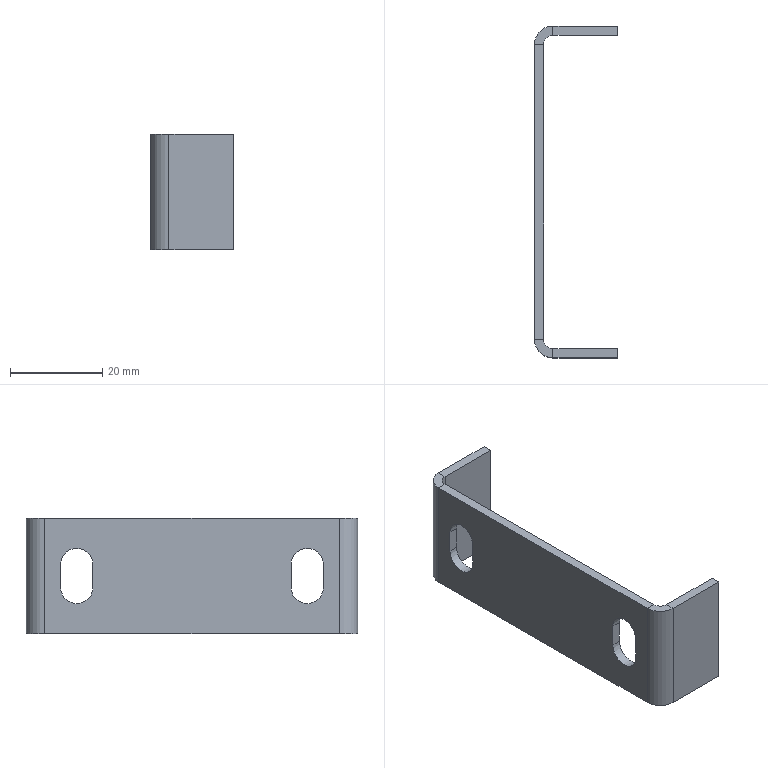Part | SolidWorks | features FlatPattern 1, ICE 1, SMBaseFlange 1, SheetMetal 1 | 1 solid | 32 faces | box 18 x 72 x 25 mm | volume 4777 mm3 | plane 22 | cylinder 10 | commonest cylinder face diameters 7 x6 4 x2 8 x2
STEP:
#1=CARTESIAN_POINT('',(2.,61.,18.5));
#2=VERTEX_POINT('',#1);
#3=CARTESIAN_POINT('',(2.,64.5,15.));
#4=VERTEX_POINT('',#3);
#5=CARTESIAN_POINT('',(2.,61.,15.));
#6=DIRECTION('',(-1.,0.,0.));
#7=DIRECTION('',(0.,0.,1.));
#8=AXIS2_PLACEMENT_3D('',#5,#6,#7);
#9=CIRCLE('',#8,3.5);
#10=EDGE_CURVE('',#2,#4,#9,.T.);
#11=ORIENTED_EDGE('',*,*,#10,.F.);
#12=CARTESIAN_POINT('',(0.,61.,18.5));
#13=VERTEX_POINT('',#12);
#14=CARTESIAN_POINT('',(2.,61.,18.5));
#15=DIRECTION('',(-1.,0.,0.));
#16=VECTOR('',#15,1000.);
#17=LINE('',#14,#16);
#18=EDGE_CURVE('',#2,#13,#17,.T.);
#19=ORIENTED_EDGE('',*,*,#18,.T.);
#20=CARTESIAN_POINT('',(0.,64.5,15.));
#21=VERTEX_POINT('',#20);
#22=CARTESIAN_POINT('',(0.,61.,15.));
#23=DIRECTION('',(-1.,0.,0.));
#24=DIRECTION('',(0.,0.,1.));
#25=AXIS2_PLACEMENT_3D('',#22,#23,#24);
#26=CIRCLE('',#25,3.5);
#27=EDGE_CURVE('',#13,#21,#26,.T.);
#28=ORIENTED_EDGE('',*,*,#27,.T.);
#29=CARTESIAN_POINT('',(2.,64.5,15.));
#30=DIRECTION('',(-1.,0.,0.));
#31=VECTOR('',#30,1000.);
#32=LINE('',#29,#31);
#33=EDGE_CURVE('',#4,#21,#32,.T.);
#34=ORIENTED_EDGE('',*,*,#33,.F.);
#35=EDGE_LOOP('',(#11,#19,#28,#34));
#36=FACE_OUTER_BOUND('',#35,.T.);
#37=CARTESIAN_POINT('',(2.,61.,15.));
#38=DIRECTION('',(-1.,0.,0.));
#39=DIRECTION('',(0.,0.,1.));
#40=AXIS2_PLACEMENT_3D('',#37,#38,#39);
#41=CYLINDRICAL_SURFACE('',#40,3.5);
#42=ADVANCED_FACE('',(#36),#41,.F.);
#43=CARTESIAN_POINT('',(2.,11.,18.5));
#44=VERTEX_POINT('',#43);
#45=CARTESIAN_POINT('',(2.,14.5,15.));
#46=VERTEX_POINT('',#45);
#47=CARTESIAN_POINT('',(2.,11.,15.));
#48=DIRECTION('',(-1.,0.,0.));
#49=DIRECTION('',(0.,0.,-1.));
#50=AXIS2_PLACEMENT_3D('',#47,#48,#49);
#51=CIRCLE('',#50,3.5);
#52=EDGE_CURVE('',#44,#46,#51,.T.);
#53=ORIENTED_EDGE('',*,*,#52,.F.);
#54=CARTESIAN_POINT('',(0.,11.,18.5));
#55=VERTEX_POINT('',#54);
#56=CARTESIAN_POINT('',(2.,11.,18.5));
#57=DIRECTION('',(-1.,0.,0.));
#58=VECTOR('',#57,1000.);
#59=LINE('',#56,#58);
#60=EDGE_CURVE('',#44,#55,#59,.T.);
#61=ORIENTED_EDGE('',*,*,#60,.T.);
#62=CARTESIAN_POINT('',(0.,14.5,15.));
#63=VERTEX_POINT('',#62);
#64=CARTESIAN_POINT('',(0.,11.,15.));
#65=DIRECTION('',(-1.,0.,0.));
#66=DIRECTION('',(0.,0.,-1.));
#67=AXIS2_PLACEMENT_3D('',#64,#65,#66);
#68=CIRCLE('',#67,3.5);
#69=EDGE_CURVE('',#55,#63,#68,.T.);
#70=ORIENTED_EDGE('',*,*,#69,.T.);
#71=CARTESIAN_POINT('',(2.,14.5,15.));
#72=DIRECTION('',(-1.,0.,0.));
#73=VECTOR('',#72,1000.);
#74=LINE('',#71,#73);
#75=EDGE_CURVE('',#46,#63,#74,.T.);
#76=ORIENTED_EDGE('',*,*,#75,.F.);
#77=EDGE_LOOP('',(#53,#61,#70,#76));
#78=FACE_OUTER_BOUND('',#77,.T.);
#79=CARTESIAN_POINT('',(2.,11.,15.));
#80=DIRECTION('',(-1.,0.,0.));
#81=DIRECTION('',(0.,0.,1.));
#82=AXIS2_PLACEMENT_3D('',#79,#80,#81);
#83=CYLINDRICAL_SURFACE('',#82,3.5);
#84=ADVANCED_FACE('',(#78),#83,.F.);
#85=CARTESIAN_POINT('',(4.,72.,25.));
#86=VERTEX_POINT('',#85);
#87=CARTESIAN_POINT('',(4.,70.,25.));
#88=VERTEX_POINT('',#87);
#89=CARTESIAN_POINT('',(4.,72.,25.));
#90=DIRECTION('',(0.,-1.,0.));
#91=VECTOR('',#90,1000.);
#92=LINE('',#89,#91);
#93=EDGE_CURVE('',#86,#88,#92,.T.);
#94=ORIENTED_EDGE('',*,*,#93,.F.);
#95=CARTESIAN_POINT('',(0.,68.,25.));
#96=VERTEX_POINT('',#95);
#97=CARTESIAN_POINT('',(4.,68.,25.));
#98=DIRECTION('',(0.,0.,-1.));
#99=DIRECTION('',(-1.,0.,0.));
#100=AXIS2_PLACEMENT_3D('',#97,#98,#99);
#101=CIRCLE('',#100,4.);
#102=EDGE_CURVE('',#96,#86,#101,.T.);
#103=ORIENTED_EDGE('',*,*,#102,.F.);
#104=CARTESIAN_POINT('',(2.,68.,25.));
#105=VERTEX_POINT('',#104);
#106=CARTESIAN_POINT('',(2.,68.,25.));
#107=DIRECTION('',(-1.,0.,0.));
#108=VECTOR('',#107,1000.);
#109=LINE('',#106,#108);
#110=EDGE_CURVE('',#105,#96,#109,.T.);
#111=ORIENTED_EDGE('',*,*,#110,.F.);
#112=CARTESIAN_POINT('',(4.,68.,25.));
#113=DIRECTION('',(0.,0.,-1.));
#114=DIRECTION('',(1.,0.,0.));
#115=AXIS2_PLACEMENT_3D('',#112,#113,#114);
#116=CIRCLE('',#115,2.);
#117=EDGE_CURVE('',#105,#88,#116,.T.);
#118=ORIENTED_EDGE('',*,*,#117,.T.);
#119=EDGE_LOOP('',(#94,#103,#111,#118));
#120=FACE_OUTER_BOUND('',#119,.T.);
#121=CARTESIAN_POINT('',(4.,72.,25.));
#122=DIRECTION('',(0.,0.,1.));
#123=DIRECTION('',(1.,0.,0.));
#124=AXIS2_PLACEMENT_3D('',#121,#122,#123);
#125=PLANE('',#124);
#126=ADVANCED_FACE('',(#120),#125,.T.);
#127=CARTESIAN_POINT('',(18.,72.,25.));
#128=VERTEX_POINT('',#127);
#129=CARTESIAN_POINT('',(0.,72.,25.));
#130=DIRECTION('',(1.,0.,0.));
#131=VECTOR('',#130,1000.);
#132=LINE('',#129,#131);
#133=EDGE_CURVE('',#86,#128,#132,.T.);
#134=ORIENTED_EDGE('',*,*,#133,.F.);
#135=ORIENTED_EDGE('',*,*,#93,.T.);
#136=CARTESIAN_POINT('',(18.,70.,25.));
#137=VERTEX_POINT('',#136);
#138=CARTESIAN_POINT('',(0.,70.,25.));
#139=DIRECTION('',(1.,0.,0.));
#140=VECTOR('',#139,1000.);
#141=LINE('',#138,#140);
#142=EDGE_CURVE('',#88,#137,#141,.T.);
#143=ORIENTED_EDGE('',*,*,#142,.T.);
#144=CARTESIAN_POINT('',(18.,72.,25.));
#145=DIRECTION('',(0.,-1.,0.));
#146=VECTOR('',#145,1000.);
#147=LINE('',#144,#146);
#148=EDGE_CURVE('',#128,#137,#147,.T.);
#149=ORIENTED_EDGE('',*,*,#148,.F.);
#150=EDGE_LOOP('',(#134,#135,#143,#149));
#151=FACE_OUTER_BOUND('',#150,.T.);
#152=CARTESIAN_POINT('',(2.,68.,25.));
#153=DIRECTION('',(0.,0.,1.));
#154=DIRECTION('',(1.,0.,0.));
#155=AXIS2_PLACEMENT_3D('',#152,#153,#154);
#156=PLANE('',#155);
#157=ADVANCED_FACE('',(#151),#156,.T.);
#158=CARTESIAN_POINT('',(0.,68.,0.));
#159=VERTEX_POINT('',#158);
#160=CARTESIAN_POINT('',(2.,68.,0.));
#161=VERTEX_POINT('',#160);
#162=CARTESIAN_POINT('',(0.,68.,0.));
#163=DIRECTION('',(1.,0.,0.));
#164=VECTOR('',#163,1000.);
#165=LINE('',#162,#164);
#166=EDGE_CURVE('',#159,#161,#165,.T.);
#167=ORIENTED_EDGE('',*,*,#166,.F.);
#168=CARTESIAN_POINT('',(4.,72.,0.));
#169=VERTEX_POINT('',#168);
#170=CARTESIAN_POINT('',(4.,68.,0.));
#171=DIRECTION('',(0.,0.,-1.));
#172=DIRECTION('',(-1.,0.,0.));
#173=AXIS2_PLACEMENT_3D('',#170,#171,#172);
#174=CIRCLE('',#173,4.);
#175=EDGE_CURVE('',#159,#169,#174,.T.);
#176=ORIENTED_EDGE('',*,*,#175,.T.);
#177=CARTESIAN_POINT('',(4.,70.,0.));
#178=VERTEX_POINT('',#177);
#179=CARTESIAN_POINT('',(4.,70.,0.));
#180=DIRECTION('',(0.,1.,0.));
#181=VECTOR('',#180,1000.);
#182=LINE('',#179,#181);
#183=EDGE_CURVE('',#178,#169,#182,.T.);
#184=ORIENTED_EDGE('',*,*,#183,.F.);
#185=CARTESIAN_POINT('',(4.,68.,0.));
#186=DIRECTION('',(0.,0.,-1.));
#187=DIRECTION('',(1.,0.,0.));
#188=AXIS2_PLACEMENT_3D('',#185,#186,#187);
#189=CIRCLE('',#188,2.);
#190=EDGE_CURVE('',#161,#178,#189,.T.);
#191=ORIENTED_EDGE('',*,*,#190,.F.);
#192=EDGE_LOOP('',(#167,#176,#184,#191));
#193=FACE_OUTER_BOUND('',#192,.T.);
#194=CARTESIAN_POINT('',(0.,68.,0.));
#195=DIRECTION('',(0.,0.,-1.));
#196=DIRECTION('',(-1.,0.,0.));
#197=AXIS2_PLACEMENT_3D('',#194,#195,#196);
#198=PLANE('',#197);
#199=ADVANCED_FACE('',(#193),#198,.T.);
#200=CARTESIAN_POINT('',(0.,4.,0.));
#201=VERTEX_POINT('',#200);
#202=CARTESIAN_POINT('',(0.,0.,0.));
#203=DIRECTION('',(0.,1.,0.));
#204=VECTOR('',#203,1000.);
#205=LINE('',#202,#204);
#206=EDGE_CURVE('',#201,#159,#205,.T.);
#207=ORIENTED_EDGE('',*,*,#206,.T.);
#208=ORIENTED_EDGE('',*,*,#166,.T.);
#209=CARTESIAN_POINT('',(2.,4.,0.));
#210=VERTEX_POINT('',#209);
#211=CARTESIAN_POINT('',(2.,0.,0.));
#212=DIRECTION('',(0.,1.,0.));
#213=VECTOR('',#212,1000.);
#214=LINE('',#211,#213);
#215=EDGE_CURVE('',#210,#161,#214,.T.);
#216=ORIENTED_EDGE('',*,*,#215,.F.);
#217=CARTESIAN_POINT('',(2.,4.,0.));
#218=DIRECTION('',(-1.,0.,0.));
#219=VECTOR('',#218,1000.);
#220=LINE('',#217,#219);
#221=EDGE_CURVE('',#210,#201,#220,.T.);
#222=ORIENTED_EDGE('',*,*,#221,.T.);
#223=EDGE_LOOP('',(#207,#208,#216,#222));
#224=FACE_OUTER_BOUND('',#223,.T.);
#225=CARTESIAN_POINT('',(4.,70.,0.));
#226=DIRECTION('',(0.,0.,-1.));
#227=DIRECTION('',(-1.,0.,0.));
#228=AXIS2_PLACEMENT_3D('',#225,#226,#227);
#229=PLANE('',#228);
#230=ADVANCED_FACE('',(#224),#229,.T.);
#231=CARTESIAN_POINT('',(0.,4.,25.));
#232=VERTEX_POINT('',#231);
#233=CARTESIAN_POINT('',(2.,4.,25.));
#234=VERTEX_POINT('',#233);
#235=CARTESIAN_POINT('',(0.,4.,25.));
#236=DIRECTION('',(1.,0.,0.));
#237=VECTOR('',#236,1000.);
#238=LINE('',#235,#237);
#239=EDGE_CURVE('',#232,#234,#238,.T.);
#240=ORIENTED_EDGE('',*,*,#239,.F.);
#241=CARTESIAN_POINT('',(4.,0.,25.));
#242=VERTEX_POINT('',#241);
#243=CARTESIAN_POINT('',(4.,4.,25.));
#244=DIRECTION('',(0.,0.,-1.));
#245=DIRECTION('',(-1.,0.,0.));
#246=AXIS2_PLACEMENT_3D('',#243,#244,#245);
#247=CIRCLE('',#246,4.);
#248=EDGE_CURVE('',#242,#232,#247,.T.);
#249=ORIENTED_EDGE('',*,*,#248,.F.);
#250=CARTESIAN_POINT('',(4.,2.,25.));
#251=VERTEX_POINT('',#250);
#252=CARTESIAN_POINT('',(4.,2.,25.));
#253=DIRECTION('',(0.,-1.,0.));
#254=VECTOR('',#253,1000.);
#255=LINE('',#252,#254);
#256=EDGE_CURVE('',#251,#242,#255,.T.);
#257=ORIENTED_EDGE('',*,*,#256,.F.);
#258=CARTESIAN_POINT('',(4.,4.,25.));
#259=DIRECTION('',(0.,0.,-1.));
#260=DIRECTION('',(1.,0.,0.));
#261=AXIS2_PLACEMENT_3D('',#258,#259,#260);
#262=CIRCLE('',#261,2.);
#263=EDGE_CURVE('',#251,#234,#262,.T.);
#264=ORIENTED_EDGE('',*,*,#263,.T.);
#265=EDGE_LOOP('',(#240,#249,#257,#264));
#266=FACE_OUTER_BOUND('',#265,.T.);
#267=CARTESIAN_POINT('',(0.,4.,25.));
#268=DIRECTION('',(0.,0.,1.));
#269=DIRECTION('',(1.,0.,0.));
#270=AXIS2_PLACEMENT_3D('',#267,#268,#269);
#271=PLANE('',#270);
#272=ADVANCED_FACE('',(#266),#271,.T.);
#273=CARTESIAN_POINT('',(0.,0.,25.));
#274=DIRECTION('',(0.,1.,0.));
#275=VECTOR('',#274,1000.);
#276=LINE('',#273,#275);
#277=EDGE_CURVE('',#232,#96,#276,.T.);
#278=ORIENTED_EDGE('',*,*,#277,.F.);
#279=ORIENTED_EDGE('',*,*,#239,.T.);
#280=CARTESIAN_POINT('',(2.,0.,25.));
#281=DIRECTION('',(0.,1.,0.));
#282=VECTOR('',#281,1000.);
#283=LINE('',#280,#282);
#284=EDGE_CURVE('',#234,#105,#283,.T.);
#285=ORIENTED_EDGE('',*,*,#284,.T.);
#286=ORIENTED_EDGE('',*,*,#110,.T.);
#287=EDGE_LOOP('',(#278,#279,#285,#286));
#288=FACE_OUTER_BOUND('',#287,.T.);
#289=CARTESIAN_POINT('',(4.,2.,25.));
#290=DIRECTION('',(0.,0.,1.));
#291=DIRECTION('',(1.,0.,0.));
#292=AXIS2_PLACEMENT_3D('',#289,#290,#291);
#293=PLANE('',#292);
#294=ADVANCED_FACE('',(#288),#293,.T.);
#295=CARTESIAN_POINT('',(4.,0.,0.));
#296=VERTEX_POINT('',#295);
#297=CARTESIAN_POINT('',(4.,2.,0.));
#298=VERTEX_POINT('',#297);
#299=CARTESIAN_POINT('',(4.,0.,0.));
#300=DIRECTION('',(0.,1.,0.));
#301=VECTOR('',#300,1000.);
#302=LINE('',#299,#301);
#303=EDGE_CURVE('',#296,#298,#302,.T.);
#304=ORIENTED_EDGE('',*,*,#303,.F.);
#305=CARTESIAN_POINT('',(4.,4.,0.));
#306=DIRECTION('',(0.,0.,-1.));
#307=DIRECTION('',(-1.,0.,0.));
#308=AXIS2_PLACEMENT_3D('',#305,#306,#307);
#309=CIRCLE('',#308,4.);
#310=EDGE_CURVE('',#296,#201,#309,.T.);
#311=ORIENTED_EDGE('',*,*,#310,.T.);
#312=ORIENTED_EDGE('',*,*,#221,.F.);
#313=CARTESIAN_POINT('',(4.,4.,0.));
#314=DIRECTION('',(0.,0.,-1.));
#315=DIRECTION('',(1.,0.,0.));
#316=AXIS2_PLACEMENT_3D('',#313,#314,#315);
#317=CIRCLE('',#316,2.);
#318=EDGE_CURVE('',#298,#210,#317,.T.);
#319=ORIENTED_EDGE('',*,*,#318,.F.);
#320=EDGE_LOOP('',(#304,#311,#312,#319));
#321=FACE_OUTER_BOUND('',#320,.T.);
#322=CARTESIAN_POINT('',(4.,0.,0.));
#323=DIRECTION('',(0.,0.,-1.));
#324=DIRECTION('',(-1.,0.,0.));
#325=AXIS2_PLACEMENT_3D('',#322,#323,#324);
#326=PLANE('',#325);
#327=ADVANCED_FACE('',(#321),#326,.T.);
#328=CARTESIAN_POINT('',(18.,0.,0.));
#329=VERTEX_POINT('',#328);
#330=CARTESIAN_POINT('',(0.,0.,0.));
#331=DIRECTION('',(-1.,0.,0.));
#332=VECTOR('',#331,1000.);
#333=LINE('',#330,#332);
#334=EDGE_CURVE('',#329,#296,#333,.T.);
#335=ORIENTED_EDGE('',*,*,#334,.T.);
#336=ORIENTED_EDGE('',*,*,#303,.T.);
#337=CARTESIAN_POINT('',(18.,2.,0.));
#338=VERTEX_POINT('',#337);
#339=CARTESIAN_POINT('',(0.,2.,0.));
#340=DIRECTION('',(-1.,0.,0.));
#341=VECTOR('',#340,1000.);
#342=LINE('',#339,#341);
#343=EDGE_CURVE('',#338,#298,#342,.T.);
#344=ORIENTED_EDGE('',*,*,#343,.F.);
#345=CARTESIAN_POINT('',(18.,2.,0.));
#346=DIRECTION('',(0.,-1.,0.));
#347=VECTOR('',#346,1000.);
#348=LINE('',#345,#347);
#349=EDGE_CURVE('',#338,#329,#348,.T.);
#350=ORIENTED_EDGE('',*,*,#349,.T.);
#351=EDGE_LOOP('',(#335,#336,#344,#350));
#352=FACE_OUTER_BOUND('',#351,.T.);
#353=CARTESIAN_POINT('',(2.,4.,0.));
#354=DIRECTION('',(0.,0.,-1.));
#355=DIRECTION('',(-1.,0.,0.));
#356=AXIS2_PLACEMENT_3D('',#353,#354,#355);
#357=PLANE('',#356);
#358=ADVANCED_FACE('',(#352),#357,.T.);
#359=CARTESIAN_POINT('',(18.,70.,0.));
#360=VERTEX_POINT('',#359);
#361=CARTESIAN_POINT('',(0.,70.,0.));
#362=DIRECTION('',(1.,0.,0.));
#363=VECTOR('',#362,1000.);
#364=LINE('',#361,#363);
#365=EDGE_CURVE('',#178,#360,#364,.T.);
#366=ORIENTED_EDGE('',*,*,#365,.T.);
#367=CARTESIAN_POINT('',(18.,70.,25.));
#368=DIRECTION('',(0.,0.,-1.));
#369=VECTOR('',#368,1000.);
#370=LINE('',#367,#369);
#371=EDGE_CURVE('',#137,#360,#370,.T.);
#372=ORIENTED_EDGE('',*,*,#371,.F.);
#373=ORIENTED_EDGE('',*,*,#142,.F.);
#374=CARTESIAN_POINT('',(4.,70.,25.));
#375=DIRECTION('',(0.,0.,-1.));
#376=VECTOR('',#375,1000.);
#377=LINE('',#374,#376);
#378=EDGE_CURVE('',#88,#178,#377,.T.);
#379=ORIENTED_EDGE('',*,*,#378,.T.);
#380=EDGE_LOOP('',(#366,#372,#373,#379));
#381=FACE_OUTER_BOUND('',#380,.T.);
#382=CARTESIAN_POINT('',(0.,70.,25.));
#383=DIRECTION('',(0.,1.,0.));
#384=DIRECTION('',(0.,0.,1.));
#385=AXIS2_PLACEMENT_3D('',#382,#383,#384);
#386=PLANE('',#385);
#387=ADVANCED_FACE('',(#381),#386,.F.);
#388=CARTESIAN_POINT('',(18.,72.,0.));
#389=VERTEX_POINT('',#388);
#390=CARTESIAN_POINT('',(18.,72.,0.));
#391=DIRECTION('',(0.,-1.,0.));
#392=VECTOR('',#391,1000.);
#393=LINE('',#390,#392);
#394=EDGE_CURVE('',#389,#360,#393,.T.);
#395=ORIENTED_EDGE('',*,*,#394,.F.);
#396=CARTESIAN_POINT('',(18.,72.,25.));
#397=DIRECTION('',(0.,0.,-1.));
#398=VECTOR('',#397,1000.);
#399=LINE('',#396,#398);
#400=EDGE_CURVE('',#128,#389,#399,.T.);
#401=ORIENTED_EDGE('',*,*,#400,.F.);
#402=ORIENTED_EDGE('',*,*,#148,.T.);
#403=ORIENTED_EDGE('',*,*,#371,.T.);
#404=EDGE_LOOP('',(#395,#401,#402,#403));
#405=FACE_OUTER_BOUND('',#404,.T.);
#406=CARTESIAN_POINT('',(18.,72.,25.));
#407=DIRECTION('',(1.,0.,0.));
#408=DIRECTION('',(0.,0.,-1.));
#409=AXIS2_PLACEMENT_3D('',#406,#407,#408);
#410=PLANE('',#409);
#411=ADVANCED_FACE('',(#405),#410,.T.);
#412=CARTESIAN_POINT('',(0.,72.,0.));
#413=DIRECTION('',(1.,0.,0.));
#414=VECTOR('',#413,1000.);
#415=LINE('',#412,#414);
#416=EDGE_CURVE('',#169,#389,#415,.T.);
#417=ORIENTED_EDGE('',*,*,#416,.F.);
#418=CARTESIAN_POINT('',(4.,72.,25.));
#419=DIRECTION('',(0.,0.,-1.));
#420=VECTOR('',#419,1000.);
#421=LINE('',#418,#420);
#422=EDGE_CURVE('',#86,#169,#421,.T.);
#423=ORIENTED_EDGE('',*,*,#422,.F.);
#424=ORIENTED_EDGE('',*,*,#133,.T.);
#425=ORIENTED_EDGE('',*,*,#400,.T.);
#426=EDGE_LOOP('',(#417,#423,#424,#425));
#427=FACE_OUTER_BOUND('',#426,.T.);
#428=CARTESIAN_POINT('',(0.,72.,25.));
#429=DIRECTION('',(0.,1.,0.));
#430=DIRECTION('',(0.,0.,1.));
#431=AXIS2_PLACEMENT_3D('',#428,#429,#430);
#432=PLANE('',#431);
#433=ADVANCED_FACE('',(#427),#432,.T.);
#434=ORIENTED_EDGE('',*,*,#175,.F.);
#435=CARTESIAN_POINT('',(0.,68.,25.));
#436=DIRECTION('',(0.,0.,-1.));
#437=VECTOR('',#436,1000.);
#438=LINE('',#435,#437);
#439=EDGE_CURVE('',#96,#159,#438,.T.);
#440=ORIENTED_EDGE('',*,*,#439,.F.);
#441=ORIENTED_EDGE('',*,*,#102,.T.);
#442=ORIENTED_EDGE('',*,*,#422,.T.);
#443=EDGE_LOOP('',(#434,#440,#441,#442));
#444=FACE_OUTER_BOUND('',#443,.T.);
#445=CARTESIAN_POINT('',(4.,68.,25.));
#446=DIRECTION('',(0.,0.,-1.));
#447=DIRECTION('',(-1.,0.,0.));
#448=AXIS2_PLACEMENT_3D('',#445,#446,#447);
#449=CYLINDRICAL_SURFACE('',#448,4.);
#450=ADVANCED_FACE('',(#444),#449,.T.);
#451=CARTESIAN_POINT('',(0.,57.5,15.));
#452=VERTEX_POINT('',#451);
#453=CARTESIAN_POINT('',(0.,61.,15.));
#454=DIRECTION('',(-1.,0.,0.));
#455=DIRECTION('',(0.,0.,1.));
#456=AXIS2_PLACEMENT_3D('',#453,#454,#455);
#457=CIRCLE('',#456,3.5);
#458=EDGE_CURVE('',#452,#13,#457,.T.);
#459=ORIENTED_EDGE('',*,*,#458,.F.);
#460=CARTESIAN_POINT('',(0.,57.5,10.));
#461=VERTEX_POINT('',#460);
#462=CARTESIAN_POINT('',(0.,57.5,15.));
#463=DIRECTION('',(0.,0.,1.));
#464=VECTOR('',#463,1000.);
#465=LINE('',#462,#464);
#466=EDGE_CURVE('',#461,#452,#465,.T.);
#467=ORIENTED_EDGE('',*,*,#466,.F.);
#468=CARTESIAN_POINT('',(0.,64.5,10.));
#469=VERTEX_POINT('',#468);
#470=CARTESIAN_POINT('',(0.,61.,10.));
#471=DIRECTION('',(-1.,0.,0.));
#472=DIRECTION('',(0.,0.,1.));
#473=AXIS2_PLACEMENT_3D('',#470,#471,#472);
#474=CIRCLE('',#473,3.5);
#475=EDGE_CURVE('',#469,#461,#474,.T.);
#476=ORIENTED_EDGE('',*,*,#475,.F.);
#477=CARTESIAN_POINT('',(0.,64.5,15.));
#478=DIRECTION('',(0.,0.,-1.));
#479=VECTOR('',#478,1000.);
#480=LINE('',#477,#479);
#481=EDGE_CURVE('',#21,#469,#480,.T.);
#482=ORIENTED_EDGE('',*,*,#481,.F.);
#483=ORIENTED_EDGE('',*,*,#27,.F.);
#484=EDGE_LOOP('',(#459,#467,#476,#482,#483));
#485=FACE_BOUND('',#484,.T.);
#486=CARTESIAN_POINT('',(0.,7.5,15.));
#487=VERTEX_POINT('',#486);
#488=CARTESIAN_POINT('',(0.,11.,15.));
#489=DIRECTION('',(-1.,0.,0.));
#490=DIRECTION('',(0.,0.,-1.));
#491=AXIS2_PLACEMENT_3D('',#488,#489,#490);
#492=CIRCLE('',#491,3.5);
#493=EDGE_CURVE('',#487,#55,#492,.T.);
#494=ORIENTED_EDGE('',*,*,#493,.F.);
#495=CARTESIAN_POINT('',(0.,7.5,10.));
#496=VERTEX_POINT('',#495);
#497=CARTESIAN_POINT('',(0.,7.5,15.));
#498=DIRECTION('',(0.,0.,1.));
#499=VECTOR('',#498,1000.);
#500=LINE('',#497,#499);
#501=EDGE_CURVE('',#496,#487,#500,.T.);
#502=ORIENTED_EDGE('',*,*,#501,.F.);
#503=CARTESIAN_POINT('',(0.,14.5,10.));
#504=VERTEX_POINT('',#503);
#505=CARTESIAN_POINT('',(0.,11.,10.));
#506=DIRECTION('',(-1.,0.,0.));
#507=DIRECTION('',(0.,0.,-1.));
#508=AXIS2_PLACEMENT_3D('',#505,#506,#507);
#509=CIRCLE('',#508,3.5);
#510=EDGE_CURVE('',#504,#496,#509,.T.);
#511=ORIENTED_EDGE('',*,*,#510,.F.);
#512=CARTESIAN_POINT('',(0.,14.5,15.));
#513=DIRECTION('',(0.,0.,-1.));
#514=VECTOR('',#513,1000.);
#515=LINE('',#512,#514);
#516=EDGE_CURVE('',#63,#504,#515,.T.);
#517=ORIENTED_EDGE('',*,*,#516,.F.);
#518=ORIENTED_EDGE('',*,*,#69,.F.);
#519=EDGE_LOOP('',(#494,#502,#511,#517,#518));
#520=FACE_BOUND('',#519,.T.);
#521=ORIENTED_EDGE('',*,*,#206,.F.);
#522=CARTESIAN_POINT('',(0.,4.,25.));
#523=DIRECTION('',(0.,0.,-1.));
#524=VECTOR('',#523,1000.);
#525=LINE('',#522,#524);
#526=EDGE_CURVE('',#232,#201,#525,.T.);
#527=ORIENTED_EDGE('',*,*,#526,.F.);
#528=ORIENTED_EDGE('',*,*,#277,.T.);
#529=ORIENTED_EDGE('',*,*,#439,.T.);
#530=EDGE_LOOP('',(#521,#527,#528,#529));
#531=FACE_OUTER_BOUND('',#530,.T.);
#532=CARTESIAN_POINT('',(0.,0.,25.));
#533=DIRECTION('',(-1.,0.,0.));
#534=DIRECTION('',(0.,0.,1.));
#535=AXIS2_PLACEMENT_3D('',#532,#533,#534);
#536=PLANE('',#535);
#537=ADVANCED_FACE('',(#485,#520,#531),#536,.T.);
#538=ORIENTED_EDGE('',*,*,#310,.F.);
#539=CARTESIAN_POINT('',(4.,0.,25.));
#540=DIRECTION('',(0.,0.,-1.));
#541=VECTOR('',#540,1000.);
#542=LINE('',#539,#541);
#543=EDGE_CURVE('',#242,#296,#542,.T.);
#544=ORIENTED_EDGE('',*,*,#543,.F.);
#545=ORIENTED_EDGE('',*,*,#248,.T.);
#546=ORIENTED_EDGE('',*,*,#526,.T.);
#547=EDGE_LOOP('',(#538,#544,#545,#546));
#548=FACE_OUTER_BOUND('',#547,.T.);
#549=CARTESIAN_POINT('',(4.,4.,25.));
#550=DIRECTION('',(0.,0.,-1.));
#551=DIRECTION('',(-1.,0.,0.));
#552=AXIS2_PLACEMENT_3D('',#549,#550,#551);
#553=CYLINDRICAL_SURFACE('',#552,4.);
#554=ADVANCED_FACE('',(#548),#553,.T.);
#555=ORIENTED_EDGE('',*,*,#334,.F.);
#556=CARTESIAN_POINT('',(18.,0.,25.));
#557=VERTEX_POINT('',#556);
#558=CARTESIAN_POINT('',(18.,0.,25.));
#559=DIRECTION('',(0.,0.,-1.));
#560=VECTOR('',#559,1000.);
#561=LINE('',#558,#560);
#562=EDGE_CURVE('',#557,#329,#561,.T.);
#563=ORIENTED_EDGE('',*,*,#562,.F.);
#564=CARTESIAN_POINT('',(0.,0.,25.));
#565=DIRECTION('',(-1.,0.,0.));
#566=VECTOR('',#565,1000.);
#567=LINE('',#564,#566);
#568=EDGE_CURVE('',#557,#242,#567,.T.);
#569=ORIENTED_EDGE('',*,*,#568,.T.);
#570=ORIENTED_EDGE('',*,*,#543,.T.);
#571=EDGE_LOOP('',(#555,#563,#569,#570));
#572=FACE_OUTER_BOUND('',#571,.T.);
#573=CARTESIAN_POINT('',(0.,0.,25.));
#574=DIRECTION('',(0.,-1.,0.));
#575=DIRECTION('',(0.,0.,-1.));
#576=AXIS2_PLACEMENT_3D('',#573,#574,#575);
#577=PLANE('',#576);
#578=ADVANCED_FACE('',(#572),#577,.T.);
#579=ORIENTED_EDGE('',*,*,#349,.F.);
#580=CARTESIAN_POINT('',(18.,2.,25.));
#581=VERTEX_POINT('',#580);
#582=CARTESIAN_POINT('',(18.,2.,25.));
#583=DIRECTION('',(0.,0.,-1.));
#584=VECTOR('',#583,1000.);
#585=LINE('',#582,#584);
#586=EDGE_CURVE('',#581,#338,#585,.T.);
#587=ORIENTED_EDGE('',*,*,#586,.F.);
#588=CARTESIAN_POINT('',(18.,2.,25.));
#589=DIRECTION('',(0.,-1.,0.));
#590=VECTOR('',#589,1000.);
#591=LINE('',#588,#590);
#592=EDGE_CURVE('',#581,#557,#591,.T.);
#593=ORIENTED_EDGE('',*,*,#592,.T.);
#594=ORIENTED_EDGE('',*,*,#562,.T.);
#595=EDGE_LOOP('',(#579,#587,#593,#594));
#596=FACE_OUTER_BOUND('',#595,.T.);
#597=CARTESIAN_POINT('',(18.,2.,25.));
#598=DIRECTION('',(1.,0.,0.));
#599=DIRECTION('',(0.,0.,-1.));
#600=AXIS2_PLACEMENT_3D('',#597,#598,#599);
#601=PLANE('',#600);
#602=ADVANCED_FACE('',(#596),#601,.T.);
#603=ORIENTED_EDGE('',*,*,#343,.T.);
#604=CARTESIAN_POINT('',(4.,2.,25.));
#605=DIRECTION('',(0.,0.,-1.));
#606=VECTOR('',#605,1000.);
#607=LINE('',#604,#606);
#608=EDGE_CURVE('',#251,#298,#607,.T.);
#609=ORIENTED_EDGE('',*,*,#608,.F.);
#610=CARTESIAN_POINT('',(0.,2.,25.));
#611=DIRECTION('',(-1.,0.,0.));
#612=VECTOR('',#611,1000.);
#613=LINE('',#610,#612);
#614=EDGE_CURVE('',#581,#251,#613,.T.);
#615=ORIENTED_EDGE('',*,*,#614,.F.);
#616=ORIENTED_EDGE('',*,*,#586,.T.);
#617=EDGE_LOOP('',(#603,#609,#615,#616));
#618=FACE_OUTER_BOUND('',#617,.T.);
#619=CARTESIAN_POINT('',(0.,2.,25.));
#620=DIRECTION('',(0.,-1.,0.));
#621=DIRECTION('',(0.,0.,-1.));
#622=AXIS2_PLACEMENT_3D('',#619,#620,#621);
#623=PLANE('',#622);
#624=ADVANCED_FACE('',(#618),#623,.F.);
#625=ORIENTED_EDGE('',*,*,#318,.T.);
#626=CARTESIAN_POINT('',(2.,4.,25.));
#627=DIRECTION('',(0.,0.,-1.));
#628=VECTOR('',#627,1000.);
#629=LINE('',#626,#628);
#630=EDGE_CURVE('',#234,#210,#629,.T.);
#631=ORIENTED_EDGE('',*,*,#630,.F.);
#632=ORIENTED_EDGE('',*,*,#263,.F.);
#633=ORIENTED_EDGE('',*,*,#608,.T.);
#634=EDGE_LOOP('',(#625,#631,#632,#633));
#635=FACE_OUTER_BOUND('',#634,.T.);
#636=CARTESIAN_POINT('',(4.,4.,25.));
#637=DIRECTION('',(0.,0.,-1.));
#638=DIRECTION('',(-1.,0.,0.));
#639=AXIS2_PLACEMENT_3D('',#636,#637,#638);
#640=CYLINDRICAL_SURFACE('',#639,2.);
#641=ADVANCED_FACE('',(#635),#640,.F.);
#642=CARTESIAN_POINT('',(2.,57.5,10.));
#643=VERTEX_POINT('',#642);
#644=CARTESIAN_POINT('',(2.,57.5,15.));
#645=VERTEX_POINT('',#644);
#646=CARTESIAN_POINT('',(2.,57.5,15.));
#647=DIRECTION('',(0.,0.,1.));
#648=VECTOR('',#647,1000.);
#649=LINE('',#646,#648);
#650=EDGE_CURVE('',#643,#645,#649,.T.);
#651=ORIENTED_EDGE('',*,*,#650,.T.);
#652=CARTESIAN_POINT('',(2.,61.,15.));
#653=DIRECTION('',(-1.,0.,0.));
#654=DIRECTION('',(0.,0.,1.));
#655=AXIS2_PLACEMENT_3D('',#652,#653,#654);
#656=CIRCLE('',#655,3.5);
#657=EDGE_CURVE('',#645,#2,#656,.T.);
#658=ORIENTED_EDGE('',*,*,#657,.T.);
#659=ORIENTED_EDGE('',*,*,#10,.T.);
#660=CARTESIAN_POINT('',(2.,64.5,10.));
#661=VERTEX_POINT('',#660);
#662=CARTESIAN_POINT('',(2.,64.5,15.));
#663=DIRECTION('',(0.,0.,-1.));
#664=VECTOR('',#663,1000.);
#665=LINE('',#662,#664);
#666=EDGE_CURVE('',#4,#661,#665,.T.);
#667=ORIENTED_EDGE('',*,*,#666,.T.);
#668=CARTESIAN_POINT('',(2.,61.,10.));
#669=DIRECTION('',(-1.,0.,0.));
#670=DIRECTION('',(0.,0.,1.));
#671=AXIS2_PLACEMENT_3D('',#668,#669,#670);
#672=CIRCLE('',#671,3.5);
#673=EDGE_CURVE('',#661,#643,#672,.T.);
#674=ORIENTED_EDGE('',*,*,#673,.T.);
#675=EDGE_LOOP('',(#651,#658,#659,#667,#674));
#676=FACE_BOUND('',#675,.T.);
#677=CARTESIAN_POINT('',(2.,7.5,10.));
#678=VERTEX_POINT('',#677);
#679=CARTESIAN_POINT('',(2.,7.5,15.));
#680=VERTEX_POINT('',#679);
#681=CARTESIAN_POINT('',(2.,7.5,15.));
#682=DIRECTION('',(0.,0.,1.));
#683=VECTOR('',#682,1000.);
#684=LINE('',#681,#683);
#685=EDGE_CURVE('',#678,#680,#684,.T.);
#686=ORIENTED_EDGE('',*,*,#685,.T.);
#687=CARTESIAN_POINT('',(2.,11.,15.));
#688=DIRECTION('',(-1.,0.,0.));
#689=DIRECTION('',(0.,0.,-1.));
#690=AXIS2_PLACEMENT_3D('',#687,#688,#689);
#691=CIRCLE('',#690,3.5);
#692=EDGE_CURVE('',#680,#44,#691,.T.);
#693=ORIENTED_EDGE('',*,*,#692,.T.);
#694=ORIENTED_EDGE('',*,*,#52,.T.);
#695=CARTESIAN_POINT('',(2.,14.5,10.));
#696=VERTEX_POINT('',#695);
#697=CARTESIAN_POINT('',(2.,14.5,15.));
#698=DIRECTION('',(0.,0.,-1.));
#699=VECTOR('',#698,1000.);
#700=LINE('',#697,#699);
#701=EDGE_CURVE('',#46,#696,#700,.T.);
#702=ORIENTED_EDGE('',*,*,#701,.T.);
#703=CARTESIAN_POINT('',(2.,11.,10.));
#704=DIRECTION('',(-1.,0.,0.));
#705=DIRECTION('',(0.,0.,-1.));
#706=AXIS2_PLACEMENT_3D('',#703,#704,#705);
#707=CIRCLE('',#706,3.5);
#708=EDGE_CURVE('',#696,#678,#707,.T.);
#709=ORIENTED_EDGE('',*,*,#708,.T.);
#710=EDGE_LOOP('',(#686,#693,#694,#702,#709));
#711=FACE_BOUND('',#710,.T.);
#712=ORIENTED_EDGE('',*,*,#215,.T.);
#713=CARTESIAN_POINT('',(2.,68.,25.));
#714=DIRECTION('',(0.,0.,-1.));
#715=VECTOR('',#714,1000.);
#716=LINE('',#713,#715);
#717=EDGE_CURVE('',#105,#161,#716,.T.);
#718=ORIENTED_EDGE('',*,*,#717,.F.);
#719=ORIENTED_EDGE('',*,*,#284,.F.);
#720=ORIENTED_EDGE('',*,*,#630,.T.);
#721=EDGE_LOOP('',(#712,#718,#719,#720));
#722=FACE_OUTER_BOUND('',#721,.T.);
#723=CARTESIAN_POINT('',(2.,0.,25.));
#724=DIRECTION('',(-1.,0.,0.));
#725=DIRECTION('',(0.,0.,1.));
#726=AXIS2_PLACEMENT_3D('',#723,#724,#725);
#727=PLANE('',#726);
#728=ADVANCED_FACE('',(#676,#711,#722),#727,.F.);
#729=ORIENTED_EDGE('',*,*,#190,.T.);
#730=ORIENTED_EDGE('',*,*,#378,.F.);
#731=ORIENTED_EDGE('',*,*,#117,.F.);
#732=ORIENTED_EDGE('',*,*,#717,.T.);
#733=EDGE_LOOP('',(#729,#730,#731,#732));
#734=FACE_OUTER_BOUND('',#733,.T.);
#735=CARTESIAN_POINT('',(4.,68.,25.));
#736=DIRECTION('',(0.,0.,-1.));
#737=DIRECTION('',(-1.,0.,0.));
#738=AXIS2_PLACEMENT_3D('',#735,#736,#737);
#739=CYLINDRICAL_SURFACE('',#738,2.);
#740=ADVANCED_FACE('',(#734),#739,.F.);
#741=ORIENTED_EDGE('',*,*,#614,.T.);
#742=ORIENTED_EDGE('',*,*,#256,.T.);
#743=ORIENTED_EDGE('',*,*,#568,.F.);
#744=ORIENTED_EDGE('',*,*,#592,.F.);
#745=EDGE_LOOP('',(#741,#742,#743,#744));
#746=FACE_OUTER_BOUND('',#745,.T.);
#747=CARTESIAN_POINT('',(4.,68.,25.));
#748=DIRECTION('',(0.,0.,-1.));
#749=DIRECTION('',(-1.,0.,0.));
#750=AXIS2_PLACEMENT_3D('',#747,#748,#749);
#751=PLANE('',#750);
#752=ADVANCED_FACE('',(#746),#751,.F.);
#753=ORIENTED_EDGE('',*,*,#365,.F.);
#754=ORIENTED_EDGE('',*,*,#183,.T.);
#755=ORIENTED_EDGE('',*,*,#416,.T.);
#756=ORIENTED_EDGE('',*,*,#394,.T.);
#757=EDGE_LOOP('',(#753,#754,#755,#756));
#758=FACE_OUTER_BOUND('',#757,.T.);
#759=CARTESIAN_POINT('',(4.,68.,0.));
#760=DIRECTION('',(0.,0.,-1.));
#761=DIRECTION('',(-1.,0.,0.));
#762=AXIS2_PLACEMENT_3D('',#759,#760,#761);
#763=PLANE('',#762);
#764=ADVANCED_FACE('',(#758),#763,.T.);
#765=ORIENTED_EDGE('',*,*,#60,.F.);
#766=ORIENTED_EDGE('',*,*,#692,.F.);
#767=CARTESIAN_POINT('',(2.,7.5,15.));
#768=DIRECTION('',(-1.,0.,0.));
#769=VECTOR('',#768,1000.);
#770=LINE('',#767,#769);
#771=EDGE_CURVE('',#680,#487,#770,.T.);
#772=ORIENTED_EDGE('',*,*,#771,.T.);
#773=ORIENTED_EDGE('',*,*,#493,.T.);
#774=EDGE_LOOP('',(#765,#766,#772,#773));
#775=FACE_OUTER_BOUND('',#774,.T.);
#776=CARTESIAN_POINT('',(2.,11.,15.));
#777=DIRECTION('',(-1.,0.,0.));
#778=DIRECTION('',(0.,0.,1.));
#779=AXIS2_PLACEMENT_3D('',#776,#777,#778);
#780=CYLINDRICAL_SURFACE('',#779,3.5);
#781=ADVANCED_FACE('',(#775),#780,.F.);
#782=ORIENTED_EDGE('',*,*,#501,.T.);
#783=ORIENTED_EDGE('',*,*,#771,.F.);
#784=ORIENTED_EDGE('',*,*,#685,.F.);
#785=CARTESIAN_POINT('',(2.,7.5,10.));
#786=DIRECTION('',(-1.,0.,0.));
#787=VECTOR('',#786,1000.);
#788=LINE('',#785,#787);
#789=EDGE_CURVE('',#678,#496,#788,.T.);
#790=ORIENTED_EDGE('',*,*,#789,.T.);
#791=EDGE_LOOP('',(#782,#783,#784,#790));
#792=FACE_OUTER_BOUND('',#791,.T.);
#793=CARTESIAN_POINT('',(2.,7.5,15.));
#794=DIRECTION('',(0.,-1.,0.));
#795=DIRECTION('',(0.,0.,-1.));
#796=AXIS2_PLACEMENT_3D('',#793,#794,#795);
#797=PLANE('',#796);
#798=ADVANCED_FACE('',(#792),#797,.F.);
#799=ORIENTED_EDGE('',*,*,#510,.T.);
#800=ORIENTED_EDGE('',*,*,#789,.F.);
#801=ORIENTED_EDGE('',*,*,#708,.F.);
#802=CARTESIAN_POINT('',(2.,14.5,10.));
#803=DIRECTION('',(-1.,0.,0.));
#804=VECTOR('',#803,1000.);
#805=LINE('',#802,#804);
#806=EDGE_CURVE('',#696,#504,#805,.T.);
#807=ORIENTED_EDGE('',*,*,#806,.T.);
#808=EDGE_LOOP('',(#799,#800,#801,#807));
#809=FACE_OUTER_BOUND('',#808,.T.);
#810=CARTESIAN_POINT('',(2.,11.,10.));
#811=DIRECTION('',(-1.,0.,0.));
#812=DIRECTION('',(0.,0.,1.));
#813=AXIS2_PLACEMENT_3D('',#810,#811,#812);
#814=CYLINDRICAL_SURFACE('',#813,3.5);
#815=ADVANCED_FACE('',(#809),#814,.F.);
#816=ORIENTED_EDGE('',*,*,#516,.T.);
#817=ORIENTED_EDGE('',*,*,#806,.F.);
#818=ORIENTED_EDGE('',*,*,#701,.F.);
#819=ORIENTED_EDGE('',*,*,#75,.T.);
#820=EDGE_LOOP('',(#816,#817,#818,#819));
#821=FACE_OUTER_BOUND('',#820,.T.);
#822=CARTESIAN_POINT('',(2.,14.5,15.));
#823=DIRECTION('',(0.,1.,0.));
#824=DIRECTION('',(0.,0.,1.));
#825=AXIS2_PLACEMENT_3D('',#822,#823,#824);
#826=PLANE('',#825);
#827=ADVANCED_FACE('',(#821),#826,.F.);
#828=ORIENTED_EDGE('',*,*,#18,.F.);
#829=ORIENTED_EDGE('',*,*,#657,.F.);
#830=CARTESIAN_POINT('',(2.,57.5,15.));
#831=DIRECTION('',(-1.,0.,0.));
#832=VECTOR('',#831,1000.);
#833=LINE('',#830,#832);
#834=EDGE_CURVE('',#645,#452,#833,.T.);
#835=ORIENTED_EDGE('',*,*,#834,.T.);
#836=ORIENTED_EDGE('',*,*,#458,.T.);
#837=EDGE_LOOP('',(#828,#829,#835,#836));
#838=FACE_OUTER_BOUND('',#837,.T.);
#839=CARTESIAN_POINT('',(2.,61.,15.));
#840=DIRECTION('',(-1.,0.,0.));
#841=DIRECTION('',(0.,0.,1.));
#842=AXIS2_PLACEMENT_3D('',#839,#840,#841);
#843=CYLINDRICAL_SURFACE('',#842,3.5);
#844=ADVANCED_FACE('',(#838),#843,.F.);
#845=ORIENTED_EDGE('',*,*,#466,.T.);
#846=ORIENTED_EDGE('',*,*,#834,.F.);
#847=ORIENTED_EDGE('',*,*,#650,.F.);
#848=CARTESIAN_POINT('',(2.,57.5,10.));
#849=DIRECTION('',(-1.,0.,0.));
#850=VECTOR('',#849,1000.);
#851=LINE('',#848,#850);
#852=EDGE_CURVE('',#643,#461,#851,.T.);
#853=ORIENTED_EDGE('',*,*,#852,.T.);
#854=EDGE_LOOP('',(#845,#846,#847,#853));
#855=FACE_OUTER_BOUND('',#854,.T.);
#856=CARTESIAN_POINT('',(2.,57.5,15.));
#857=DIRECTION('',(0.,-1.,0.));
#858=DIRECTION('',(0.,0.,-1.));
#859=AXIS2_PLACEMENT_3D('',#856,#857,#858);
#860=PLANE('',#859);
#861=ADVANCED_FACE('',(#855),#860,.F.);
#862=ORIENTED_EDGE('',*,*,#475,.T.);
#863=ORIENTED_EDGE('',*,*,#852,.F.);
#864=ORIENTED_EDGE('',*,*,#673,.F.);
#865=CARTESIAN_POINT('',(2.,64.5,10.));
#866=DIRECTION('',(-1.,0.,0.));
#867=VECTOR('',#866,1000.);
#868=LINE('',#865,#867);
#869=EDGE_CURVE('',#661,#469,#868,.T.);
#870=ORIENTED_EDGE('',*,*,#869,.T.);
#871=EDGE_LOOP('',(#862,#863,#864,#870));
#872=FACE_OUTER_BOUND('',#871,.T.);
#873=CARTESIAN_POINT('',(2.,61.,10.));
#874=DIRECTION('',(-1.,0.,0.));
#875=DIRECTION('',(0.,0.,1.));
#876=AXIS2_PLACEMENT_3D('',#873,#874,#875);
#877=CYLINDRICAL_SURFACE('',#876,3.5);
#878=ADVANCED_FACE('',(#872),#877,.F.);
#879=ORIENTED_EDGE('',*,*,#481,.T.);
#880=ORIENTED_EDGE('',*,*,#869,.F.);
#881=ORIENTED_EDGE('',*,*,#666,.F.);
#882=ORIENTED_EDGE('',*,*,#33,.T.);
#883=EDGE_LOOP('',(#879,#880,#881,#882));
#884=FACE_OUTER_BOUND('',#883,.T.);
#885=CARTESIAN_POINT('',(2.,64.5,15.));
#886=DIRECTION('',(0.,1.,0.));
#887=DIRECTION('',(0.,0.,1.));
#888=AXIS2_PLACEMENT_3D('',#885,#886,#887);
#889=PLANE('',#888);
#890=ADVANCED_FACE('',(#884),#889,.F.);
#891=CLOSED_SHELL('',(#42,#84,#126,#157,#199,#230,#272,#294,#327,#358,#387,#411,#433,#450,#537,#554,#578,#602,#624,#641,#728,#740,#752,#764,#781,#798,#815,#827,#844,#861,#878,#890));
#892=MANIFOLD_SOLID_BREP('',#891);
#893=CARTESIAN_POINT('',(0.,0.,0.));
#894=DIRECTION('',(0.,0.,1.));
#895=DIRECTION('',(1.,0.,0.));
#896=AXIS2_PLACEMENT_3D('',#893,#894,#895);
#897=(LENGTH_UNIT()NAMED_UNIT(*)SI_UNIT(.MILLI.,.METRE.));
#898=UNCERTAINTY_MEASURE_WITH_UNIT(LENGTH_MEASURE(0.00001),#897,'','');
#899=(NAMED_UNIT(*)PLANE_ANGLE_UNIT()SI_UNIT($,.RADIAN.));
#900=(NAMED_UNIT(*)SI_UNIT($,.STERADIAN.)SOLID_ANGLE_UNIT());
#901=(GEOMETRIC_REPRESENTATION_CONTEXT(3)GLOBAL_UNCERTAINTY_ASSIGNED_CONTEXT((#898))GLOBAL_UNIT_ASSIGNED_CONTEXT((#897,#899,#900))REPRESENTATION_CONTEXT('',''));
#902=ADVANCED_BREP_SHAPE_REPRESENTATION('',(#892,#896),#901);